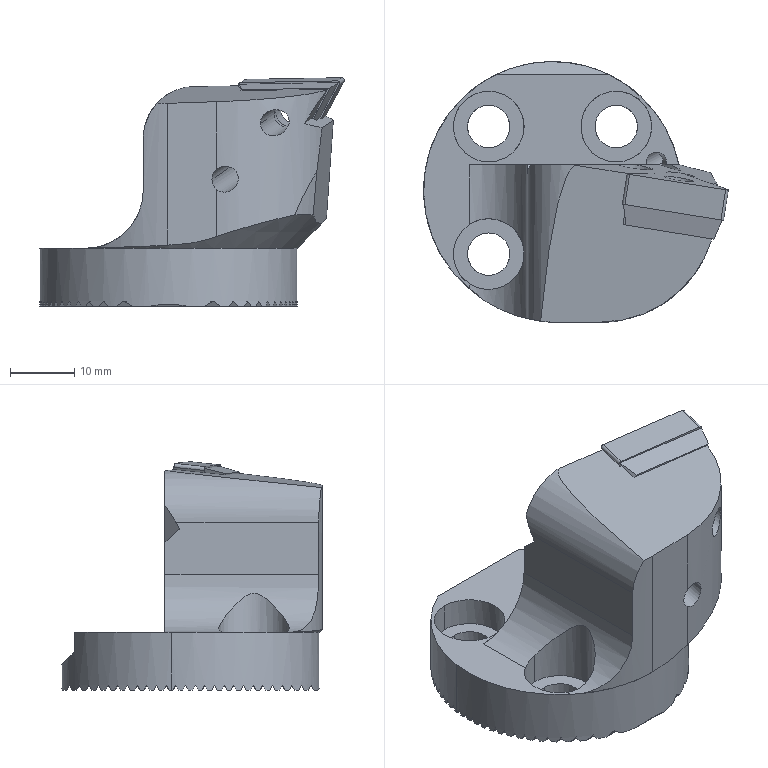NC program | Mastercam | posted with a generic post
Lines 6760 to 8002 of 11065:
(6 FEMR |TOOL - 5|DIA. OFF. - 5|LEN. - 5|TOOL DIA. - 6.)
N3668 T5 M6
N3670 G0 G54 G90 X39.195 Y22.78 C9. B-84. S3500 M3
N3672 G43 H5 Z49.995
N3674 Z1.995
N3676 G1 Z.245 F2000.
N3678 X38.335 Y23.239 Z.094 F1500.
N3680 G3 X37.724 Y23.398 Z-.005 I-.635 J-1.191
N3682 G1 X37.408 Y23.403
N3684 X37.341 Y23.163
N3686 G3 X37.182 Y21.033 I16.83 J-2.327
N3688 X37.053 Y14.522 I744.923 J-18.08
N3690 G1 X37.263 Y14.518
N3692 X37.474 Y14.514
N3694 X37.497 Z-.002
N3696 G3 X38.823 Y15.607 Z.245 J1.35
N3698 X38.847 Y15.825 I-1.326 J.257
N3700 G1 X39.026 Y22.009 F9500.
N3702 G3 X39.027 Y22.048 I-1.349 J.039
N3704 X39.01 Y22.26 I-1.35
N3706 X37.7 Y23.398 Z-.005 I-1.333 J-.212 F1500.
N3708 G1 X37.385 Y23.404
N3710 X37.365
N3712 G3 X37.157 Y22.633 I2.482 J-1.081
N3714 X36.967 Y20.031 I22.315 J-2.94
N3716 X36.875 Y15.018 I225.707 J-6.634
N3718 X36.908 Y14.704 I5.723 J.429
N3720 G1 X36.925 Y14.524
N3722 X37.346 Y14.517
N3724 X37.369 Z-.002
N3726 X37.633 Y14.543 Z.033
N3728 X37.887 Y14.62 Z.069
N3730 X38.121 Y14.746 Z.104
N3732 X38.326 Y14.915 Z.139
N3734 X38.493 Y15.12 Z.174
N3736 X38.618 Y15.355 Z.21
N3738 X38.694 Y15.609 Z.245
N3740 G3 X38.718 Y15.809 I-1.326 J.257 F9500.
N3742 G1 X38.98 Y21.992
N3744 G3 X38.981 Y22.049 I-1.348 J.057
N3746 X38.965 Y22.26 I-1.349
N3748 X37.655 Y23.399 Z-.005 I-1.333 J-.211 F1500.
N3750 G1 X37.339 Y23.404
N3752 X37.314 Y23.405
N3754 G3 X37.029 Y22.547 I2.55 J-1.324
N3756 X36.784 Y20.027 I17.143 J-2.938
N3758 X36.693 Y15.501 I112.328 J-4.526
N3760 G1 Y15.409
N3762 G3 X36.807 Y14.526 I4.202 J.095
N3764 G1 X37.018 Y14.522
N3766 X37.228 Y14.519
N3768 X37.252 Z-.002
N3770 G3 X38.577 Y15.611 Z.245 J1.35
N3772 X38.6 Y15.797 I-1.325 J.258 F9500.
N3774 G1 X38.926 Y21.979
N3776 G3 X38.928 Y22.05 I-1.349 J.071
N3778 X38.911 Y22.261 I-1.351
N3780 X37.601 Y23.4 Z-.005 I-1.334 J-.211 F1500.
N3782 G1 X37.285 Y23.405
N3784 X37.256 Y23.406
N3786 G3 X36.928 Y22.594 I2.236 J-1.377
N3788 X36.626 Y20.376 I12.079 J-2.771
N3790 X36.503 Y16.145 I72.788 J-4.231
N3792 X36.504 Y15.803 I72.911
N3794 X36.694 Y14.528 I4.559 J.028
N3796 G1 X36.905 Y14.524
N3798 X37.115 Y14.521
N3800 X37.139 Z-.002
N3802 G3 X38.464 Y15.613 Z.245 J1.349
N3804 X38.486 Y15.788 I-1.325 J.257 F9500.
N3806 G1 X38.865 Y21.968
N3808 G3 X38.868 Y22.051 I-1.347 J.083
N3810 X38.851 Y22.262 I-1.35
N3812 X37.542 Y23.401 Z-.005 I-1.333 J-.211 F1500.
N3814 G1 X37.226 Y23.406
N3816 X37.194 Y23.407
N3818 G3 X36.83 Y22.633 I2.017 J-1.424
N3820 X36.466 Y20.502 I9.938 J-2.789
N3822 X36.318 Y16.715 I48.508 J-3.787
N3824 X36.324 Y16.008 I48.656
N3826 X36.49 Y14.817 I5.524 J.16
N3828 G2 X36.584 Y14.53 I-6.781 J-2.398
N3830 G1 X36.795 Y14.526
N3832 X37.005 Y14.523
N3834 X37.029 Z-.002
N3836 G3 X38.354 Y15.615 Z.245 J1.349
N3838 X38.375 Y15.779 I-1.325 J.257 F9500.
N3840 G1 X38.802 Y21.959
N3842 G3 X38.805 Y22.052 I-1.347 J.093
N3844 X38.788 Y22.263 I-1.35
N3846 X37.479 Y23.402 Z-.005 I-1.333 J-.211 F1500.
N3848 G1 X37.163 Y23.408
N3850 X37.129
N3852 G3 X36.733 Y22.669 I1.839 J-1.46
N3854 X36.312 Y20.613 I8.505 J-2.813
N3856 X36.134 Y17.034 I35.883 J-3.579
N3858 X36.144 Y16.196 I36.061
N3860 X36.381 Y14.772 I5.219 J.137
N3862 G1 X36.476 Y14.532
N3864 X36.897 Y14.525
N3866 X36.92 Y14.524 Z-.002
N3868 G3 X38.246 Y15.617 Z.245 J1.35
N3870 X38.267 Y15.772 I-1.326 J.257 F9500.
N3872 G1 X38.735 Y21.951
N3874 G3 X38.739 Y22.053 I-1.346 J.102
N3876 X38.722 Y22.265 I-1.35
N3878 X37.413 Y23.403 Z-.005 I-1.333 J-.212 F1500.
N3880 G1 X37.097 Y23.409
N3882 X37.061
N3884 G3 X36.639 Y22.702 I1.685 J-1.485
N3886 X36.164 Y20.713 I7.489 J-2.841
N3888 X35.954 Y17.323 I27.281 J-3.39
N3890 X35.977 Y16.2 I27.491
N3892 X36.253 Y14.788 I4.982 J.242
N3894 G2 X36.368 Y14.534 I-8.619 J-4.061
N3896 G1 X36.579 Y14.53
N3898 X36.789 Y14.526
N3900 X36.813 Z-.002
N3902 G3 X38.138 Y15.619 Z.245 J1.35
N3904 X38.158 Y15.766 I-1.325 J.257 F9500.
N3906 G1 X38.666 Y21.944
N3908 G3 X38.671 Y22.055 I-1.345 J.111
N3910 X38.654 Y22.266 I-1.35
N3912 X37.344 Y23.404 Z-.005 I-1.333 J-.211 F1500.
N3914 G1 X37.029 Y23.41
N3916 X36.991 Y23.411
N3918 G3 X36.545 Y22.733 I1.555 J-1.509
N3920 X36.02 Y20.805 I6.732 J-2.872
N3922 X35.775 Y17.456 I22.746 J-3.349
N3924 X35.801 Y16.362 I22.991
N3926 X36.127 Y14.801 I4.97 J.225
N3928 X36.262 Y14.536 I5.706 J2.736
N3930 G1 X36.472 Y14.532
N3932 X36.683 Y14.528
N3934 X36.706 Z-.002
N3936 G3 X38.032 Y15.62 Z.245 J1.35
N3938 X38.051 Y15.76 I-1.326 J.258 F9500.
N3940 G1 X38.595 Y21.937
N3942 G3 X38.6 Y22.056 I-1.345 J.119
N3944 X38.584 Y22.267 I-1.35
N3946 X37.274 Y23.406 Z-.005 I-1.334 J-.211 F1500.
N3948 G1 X36.958 Y23.411
N3950 X36.919 Y23.412
N3952 G3 X36.453 Y22.763 I1.444 J-1.529
N3954 X35.88 Y20.891 I6.133 J-2.903
N3956 X35.6 Y17.599 I19.196 J-3.292
N3958 X35.639 Y16.351 I19.476
N3960 X36.002 Y14.812 I4.768 J.311
N3962 X36.039 Y14.74 I1.147 J.55
N3964 X36.225 Y14.536 I.525 J.292
N3966 G1 X36.436 Y14.533
N3968 X36.459 Z-.002
N3970 G3 X37.784 Y15.625 Z.245 J1.349
N3972 X37.8 Y15.726 I-1.325 J.257 F9500.
N3974 G1 X38.519 Y21.901
N3976 G3 X38.528 Y22.057 I-1.341 J.156
N3978 X38.512 Y22.268 I-1.35
N3980 X37.202 Y23.407 Z-.005 I-1.334 J-.211 F1500.
N3982 G1 X36.886 Y23.412
N3984 X36.845 Y23.413
N3986 G3 X36.361 Y22.792 I1.332 J-1.536
N3988 X35.743 Y20.973 I5.644 J-2.932
N3990 X35.425 Y17.675 I16.95 J-3.298
N3992 X35.466 Y16.496 I17.268
N3994 X35.82 Y14.952 I4.95 J.325
N3996 X35.95 Y14.731 I1.379 J.659
N3998 X36.162 Y14.537 I.499 J.333
N4000 G1 X36.372 Y14.534
N4002 X36.396 Z-.002
N4004 G3 X37.721 Y15.626 Z.245 J1.349
N4006 X37.737 Y15.73 I-1.325 J.257 F9500.
N4008 G1 X38.445 Y21.904
N4010 G3 X38.454 Y22.058 I-1.341 J.154
N4012 X38.438 Y22.27 I-1.35
N4014 X37.128 Y23.408 Z-.005 I-1.334 J-.212 F1500.
N4016 G1 X36.812 Y23.414
N4018 X36.769
N4020 G3 X36.208 Y22.715 I1.314 J-1.627
N4022 X35.539 Y20.717 I6.131 J-3.164
N4024 X35.255 Y17.774 I15.082 J-2.943
N4026 X35.31 Y16.474 I15.366
N4028 X35.652 Y15.063 I4.788 J.415
N4030 X35.99 Y14.606 I.996 J.383
N4032 X36.128 Y14.538 I.331 J.5
N4034 G1 X36.137 Y14.566 Z-.001
N4036 X36.682 Y16.34 Z.245
N4038 X38.319 Y21.663 F9500.
N4040 G3 X38.379 Y22.06 I-1.29 J.397
N4042 X38.362 Y22.271 I-1.35
N4044 X37.052 Y23.409 Z-.005 I-1.333 J-.211 F1500.
N4046 G1 X36.736 Y23.415
N4048 X36.691 Y23.416
N4050 G3 X36.115 Y22.746 I1.208 J-1.623
N4052 X35.403 Y20.799 I5.691 J-3.183
N4054 X35.087 Y17.845 I13.643 J-2.954
N4056 X35.157 Y16.449 I13.959
N4058 X35.569 Y14.999 I4.139 J.391
N4060 X35.898 Y14.611 I.953 J.474
N4062 X36.073 Y14.539 I.312 J.512
N4064 G2 X36.104 Y14.661 Z.012 I1.322 J-.272
N4066 G1 X36.618 Y16.343 Z.245
N4068 X38.242 Y21.667 F9500.
N4070 G3 X38.301 Y22.061 I-1.291 J.394
N4072 X38.285 Y22.272 I-1.35
N4074 X36.975 Y23.411 Z-.005 I-1.334 J-.211 F1500.
N4076 G1 X36.659 Y23.416
N4078 X36.612 Y23.417
N4080 G3 X36.022 Y22.777 I1.245 J-1.739
N4082 X35.27 Y20.878 I5.309 J-3.2
N4084 X34.921 Y17.884 I12.673 J-2.994
N4086 X34.987 Y16.578 I13.022
N4088 X35.401 Y15.092 I4.356 J.414
N4090 X35.81 Y14.605 I1.088 J.497
N4092 X35.98 Y14.541 I.294 J.523
N4094 G2 X36.017 Y14.689 Z.016 I1.327 J-.249
N4096 G1 X36.526 Y16.344 Z.245
N4098 X38.163 Y21.665 F9500.
N4100 G3 X38.223 Y22.062 I-1.291 J.397
N4102 X38.206 Y22.274 I-1.351
N4104 X36.896 Y23.412 Z-.005 I-1.334 J-.212 F1500.
N4106 G1 X36.58 Y23.418
N4108 X36.531 Y23.419
N4110 G3 X35.861 Y22.706 I1.286 J-1.879
N4112 X35.099 Y20.794 I5.44 J-3.276
N4114 X34.757 Y17.944 I11.709 J-2.85
N4116 X34.838 Y16.55 I12.051
N4118 X35.281 Y15.094 I4.178 J.474
N4120 X35.722 Y14.595 I1.105 J.533
N4122 X35.867 Y14.542 I.276 J.533
N4124 G2 X35.903 Y14.684 Z.015 I1.324 J-.26
N4126 G1 X36.421 Y16.344 Z.245
N4128 X38.081 Y21.662 F9500.
N4130 G3 X38.142 Y22.064 I-1.289 J.402
N4132 X38.125 Y22.275 I-1.35
N4134 X36.816 Y23.414 Z-.005 I-1.333 J-.211 F1500.
N4136 G1 X36.5 Y23.419
N4138 X36.448 Y23.42
N4140 G3 X35.698 Y22.636 I1.335 J-2.027
N4142 X34.89 Y20.549 I5.681 J-3.402
N4144 X34.596 Y17.978 I11.096 J-2.571
N4146 X34.671 Y16.67 I11.39
N4148 X35.163 Y15.089 I4.304 J.473
N4150 X35.626 Y14.594 I1.103 J.566
N4152 X35.79 Y14.544 I.254 J.543
N4154 G2 X35.839 Y14.762 Z.025 I1.337 J-.185
N4156 G1 X36.335 Y16.347 Z.245
N4158 X37.998 Y21.662 F9500.
N4160 G3 X38.06 Y22.065 I-1.288 J.403
N4162 X38.043 Y22.276 I-1.35
N4164 X36.734 Y23.415 Z-.005 I-1.333 J-.211 F1500.
N4166 G1 X36.418 Y23.421
N4168 X36.364
N4170 G3 X35.602 Y22.671 I1.302 J-2.084
N4172 X34.757 Y20.63 I5.341 J-3.407
N4174 X34.435 Y18.029 I10.353 J-2.601
N4176 X34.526 Y16.636 I10.675
N4178 X35.049 Y15.077 I4.19 J.536
N4180 X35.529 Y14.59 I1.115 J.621
N4182 X35.698 Y14.545 I.236 J.552
N4184 G2 X35.754 Y14.813 Z.032 I1.343 J-.138
N4186 G1 X36.238 Y16.35 Z.245
N4188 X37.914 Y21.66 F9500.
N4190 G3 X37.977 Y22.067 I-1.287 J.407
N4192 X37.96 Y22.278 I-1.35
N4194 X36.65 Y23.416 Z-.005 I-1.333 J-.211 F1500.
N4196 G1 X36.334 Y23.422
N4198 X36.278 Y23.423
N4200 G3 X35.506 Y22.705 I1.218 J-2.085
N4202 X34.627 Y20.71 I5.032 J-3.408
N4204 X34.278 Y18.056 I9.904 J-2.654
N4206 X34.361 Y16.748 I10.253
N4208 X34.881 Y15.148 I4.427 J.553
N4210 X35.259 Y14.689 I1.565 J.907
N4212 X35.549 Y14.548 I.398 J.449
N4214 G2 X35.597 Y14.746 Z.022 I1.332 J-.217
N4216 G1 X36.113 Y16.346 Z.245
N4218 X37.826 Y21.653 F9500.
N4220 G3 X37.891 Y22.068 I-1.284 J.415
N4222 X37.875 Y22.279 I-1.349
N4224 X36.565 Y23.418 Z-.005 I-1.333 J-.211 F1500.
N4226 G1 X36.249 Y23.423
N4228 X36.19 Y23.424
N4230 G3 X35.337 Y22.64 I1.223 J-2.187
N4232 X34.456 Y20.63 I5.151 J-3.455
N4234 X34.12 Y18.098 I9.386 J-2.532
N4236 X34.22 Y16.707 I9.722
N4238 X34.766 Y15.13 I4.322 J.613
N4240 X35.143 Y14.689 I1.556 J.949
N4242 X35.481 Y14.549 I.388 J.458
N4244 G2 X35.543 Y14.863 Z.038 I1.347 J-.101
N4246 G1 X36.024 Y16.352 Z.245
N4248 X37.739 Y21.654 F9500.
N4250 G3 X37.805 Y22.07 I-1.284 J.416
N4252 X37.788 Y22.281 I-1.35
N4254 X36.478 Y23.419 Z-.005 I-1.333 J-.211 F1500.
N4256 G1 X36.163 Y23.425
N4258 X36.101 Y23.426
N4260 G3 X35.239 Y22.676 I1.109 J-2.145
N4262 X34.327 Y20.707 I4.888 J-3.459
N4264 X33.966 Y18.118 I9.105 J-2.589
N4266 X34.057 Y16.811 I9.466
N4268 X34.653 Y15.11 I4.342 J.566
N4270 X35.048 Y14.673 I1.413 J.88
N4272 X35.4 Y14.551 I.362 J.478
N4274 G1 X35.423 Z-.002
N4276 X35.687 Y14.577 Z.033
N4278 X35.941 Y14.654 Z.069
N4280 X36.175 Y14.78 Z.104
N4282 X36.38 Y14.949 Z.139
N4284 X36.547 Y15.154 Z.174
N4286 X36.672 Y15.389 Z.21
N4288 X36.748 Y15.643 Z.245
N4290 G3 X36.758 Y15.696 I-1.326 J.257 F9500.
N4292 G1 X37.701 Y21.867
N4294 G3 X37.717 Y22.071 I-1.334 J.204
N4296 X37.7 Y22.282 I-1.35
N4298 X36.39 Y23.421 Z-.005 I-1.333 J-.211 F1500.
N4300 G1 X36.075 Y23.427
N4302 X36.01 Y23.428
N4304 G3 X35.141 Y22.71 I1.012 J-2.111
N4306 X34.2 Y20.781 I4.654 J-3.463
N4308 X33.812 Y18.151 I8.73 J-2.63
N4310 X33.919 Y16.763 I9.118
N4312 X34.541 Y15.087 I4.244 J.621
N4314 X34.923 Y14.677 I1.437 J.957
N4316 X35.278 Y14.553 I.366 J.476
N4318 G1 X35.302 Z-.002
N4320 G3 X36.627 Y15.645 Z.245 J1.35
N4322 X36.635 Y15.692 I-1.325 J.258 F9500.
N4324 G1 X37.61 Y21.862
N4326 G3 X37.627 Y22.073 I-1.333 J.211
N4328 X37.61 Y22.284 I-1.35
N4330 X36.3 Y23.423 Z-.005 I-1.333 J-.211 F1500.
N4332 G1 X35.985 Y23.428
N4334 X35.857 Y23.407
N4336 G3 X34.89 Y22.547 I1.237 J-2.364
N4338 X33.943 Y20.389 I5.295 J-3.609
N4340 X33.657 Y18.182 I8.386 J-2.207
N4342 X33.783 Y16.712 I8.672
N4344 X34.43 Y15.062 I4.142 J.673
N4346 X34.809 Y14.672 I1.396 J.974
N4348 X35.154 Y14.555 I.355 J.483
N4350 G1 X35.364 Y14.551
N4352 X35.388 Z-.002
N4354 G3 X36.713 Y15.643 Z.245 J1.35
N4356 X36.727 Y15.728 I-1.325 J.258 F9500.
N4358 G1 X37.524 Y21.901
N4360 G3 X37.535 Y22.074 I-1.339 J.173
N4362 X37.519 Y22.286 I-1.35
N4364 X36.209 Y23.424 Z-.005 I-1.334 J-.212 F1500.
N4366 G1 X35.893 Y23.43
N4368 X35.763 Y23.411
N4370 G3 X34.788 Y22.584 I1.13 J-2.322
N4372 X33.813 Y20.464 I5.056 J-3.608
N4374 X33.508 Y18.206 I8.192 J-2.258
N4376 X33.65 Y16.657 I8.497
N4378 X34.322 Y15.035 I4.041 J.723
N4380 X34.692 Y14.667 I1.342 J.979
N4382 X35.028 Y14.557 I.346 J.49
N4384 G1 X35.238 Y14.553
N4386 X35.262 Z-.002
N4388 G3 X36.587 Y15.646 Z.245 J1.35
N4390 X36.6 Y15.723 I-1.325 J.257 F9500.
N4392 G1 X37.43 Y21.896
N4394 G3 X37.442 Y22.076 I-1.338 J.18
N4396 X37.426 Y22.287 I-1.35
N4398 X36.116 Y23.426 Z-.005 I-1.334 J-.211 F1500.
N4400 G1 X35.8 Y23.431
N4402 X35.666 Y23.414
N4404 G3 X34.685 Y22.619 I1.03 J-2.274
N4406 X33.684 Y20.534 I4.836 J-3.604
N4408 X33.358 Y18.23 I7.983 J-2.304
N4410 X33.52 Y16.599 I8.309
N4412 X34.215 Y15.006 I3.936 J.769
N4414 X34.842 Y14.569 I.945 J.689
N4416 X35.063 Y14.552 I.221 J1.406
N4418 X35.155 Y14.555 J1.423
N4420 G1 X35.179 Z-.002
N4422 G3 X36.504 Y15.647 Z.245 J1.35
N4424 X36.517 Y15.727 I-1.325 J.258 F9500.
N4426 G1 X37.336 Y21.9
N4428 G3 X37.348 Y22.078 I-1.338 J.178
N4430 X37.331 Y22.289 I-1.35
N4432 X36.021 Y23.427 Z-.005 I-1.333 J-.211 F1500.
N4434 G1 X35.706 Y23.433
N4436 X35.567 Y23.417
N4438 G3 X34.58 Y22.651 I.957 J-2.253
N4440 X33.555 Y20.6 I4.636 J-3.597
N4442 X33.206 Y18.247 I7.769 J-2.353
N4444 X33.359 Y16.68 I8.118
N4446 X34.04 Y15.063 I4.103 J.775
N4448 X34.215 Y14.903 I.484 J.354
N4450 G1 X34.396 Y14.794
N4452 G3 X34.842 Y14.569 I.899 J1.226
N4454 X34.955 Y14.558 Z.01 I.113 J.589
N4456 X35.548 Y15.068 Z.123 J.6
N4458 G1 X35.687 Y15.977 Z.245
N4460 X36.607 Y21.987 F9500.
N4462 X36.689 Y22.523 Z.173 F1500.
N4464 G3 X36.698 Y22.642 Z.157 I-.778 J.119
N4466 X35.925 Y23.429 Z-.005 I-.787
N4468 G1 X35.609 Y23.435
N4470 X35.465 Y23.42
N4472 G3 X34.473 Y22.681 I.887 J-2.225
N4474 X33.427 Y20.661 I4.426 J-3.574
N4476 X33.06 Y18.266 I7.623 J-2.395
N4478 X33.232 Y16.612 I7.99
N4480 X33.813 Y15.202 I4.108 J.869
N4482 X33.992 Y15.037 I.488 J.349
N4484 G1 X34.173 Y14.928
N4486 X34.353 Y14.82
N4488 G3 X35.049 Y14.627 Z.092 I.696 J1.157
N4490 X36.067 Y15.092 Z.245 J1.35
N4492 X36.388 Y15.812 I-1.018 J.885 F9500.
N4494 G1 X37.142 Y21.916
N4496 G3 X37.152 Y22.081 I-1.34 J.165
N4498 X37.135 Y22.292 I-1.35
N4500 X35.825 Y23.431 Z-.005 I-1.333 J-.211 F1500.
N4502 G1 X35.51 Y23.436
N4504 X35.362 Y23.423
N4506 G3 X34.367 Y22.711 I.821 J-2.198
N4508 X33.299 Y20.721 I4.267 J-3.572
N4510 X32.912 Y18.275 I7.542 J-2.446
N4512 X33.073 Y16.685 I7.929
N4514 X33.598 Y15.341 I4.076 J.817
N4516 X33.788 Y15.16 I.499 J.333
N4518 G1 X33.969 Y15.051
N4520 X34.149 Y14.943
N4522 G3 X34.844 Y14.75 Z.092 I.695 J1.157
N4524 X35.863 Y15.214 Z.245 J1.35
N4526 X36.181 Y15.909 I-1.019 J.886 F9500.
N4528 G1 X37.036 Y21.892
N4530 G3 X37.05 Y22.083 I-1.336 J.191
N4532 X37.033 Y22.294 I-1.35
N4534 X35.723 Y23.433 Z-.005 I-1.333 J-.211 F1500.
N4536 G1 X35.408 Y23.438
N4538 X35.257 Y23.427
N4540 G3 X34.261 Y22.741 I.758 J-2.169
N4542 X33.172 Y20.78 I4.134 J-3.578
N4544 X32.764 Y18.294 I7.376 J-2.486
N4546 X32.948 Y16.614 I7.784
N4548 X33.405 Y15.458 I3.742 J.811
N4550 X33.596 Y15.275 I.5 J.332
N4552 G1 X33.776 Y15.167
N4554 X33.956 Y15.058
N4556 G3 X34.652 Y14.865 Z.092 I.696 J1.158
N4558 X35.671 Y15.33 Z.245 J1.351
N4560 X35.985 Y16.001 I-1.019 J.886 F9500.
N4562 G1 X36.929 Y21.87
N4564 G3 X36.946 Y22.085 I-1.333 J.215
N4566 X36.929 Y22.296 I-1.35
N4568 X35.62 Y23.434 Z-.005 I-1.333 J-.211 F1500.
N4570 G1 X35.304 Y23.44
N4572 X35.149 Y23.43
N4574 G3 X34.15 Y22.767 I.702 J-2.141
N4576 X33.044 Y20.832 I4.009 J-3.577
N4578 X32.618 Y18.311 I7.245 J-2.521
N4580 X32.825 Y16.538 I7.671
N4582 X33.209 Y15.585 I3.395 J.813
N4584 X33.41 Y15.387 I.51 J.316
N4586 G1 X33.591 Y15.278
N4588 X33.771 Y15.17
N4590 G3 X34.466 Y14.977 Z.092 I.695 J1.157
N4592 X35.485 Y15.441 Z.245 J1.35
N4594 X35.795 Y16.091 I-1.019 J.886 F9500.
N4596 G1 X36.82 Y21.85
N4598 G3 X36.841 Y22.087 I-1.33 J.237
N4600 X36.824 Y22.298 I-1.351
N4602 X35.514 Y23.436 Z-.005 I-1.334 J-.211 F1500.
N4604 G1 X35.198 Y23.442
N4606 X34.992 Y23.42
N4608 G3 X33.977 Y22.726 I.778 J-2.227
N4610 X32.83 Y20.623 I4.142 J-3.625
N4612 X32.473 Y18.317 I7.268 J-2.306
N4614 X32.66 Y16.634 I7.625
N4616 X33.028 Y15.695 I3.285 J.746
N4618 X33.231 Y15.494 I.512 J.314
N4620 G1 X33.411 Y15.386
N4622 X33.592 Y15.278
N4624 G3 X34.287 Y15.085 Z.092 I.695 J1.157
N4626 X35.306 Y15.549 Z.245 J1.35
N4628 X35.612 Y16.177 I-1.019 J.886 F9500.
N4630 G1 X36.712 Y21.83
N4632 G3 X36.737 Y22.088 I-1.325 J.258
N4634 X36.721 Y22.299 I-1.35
N4636 X35.411 Y23.438 Z-.005 I-1.334 J-.211 F1500.
N4638 X35.095 Y23.444 I-.876 J-41.251
N4640 G1 X35.089
N4642 G3 X34.798 Y23.368 J-.6
N4644 G1 X34.614 Y23.266
N4646 G3 X33.509 Y22.311 I1.244 J-2.557
N4648 X32.457 Y19.71 I5.355 J-3.678
N4650 X32.327 Y18.33 I7.285 J-1.38
N4652 X32.55 Y16.528 I7.415
N4654 X32.858 Y15.794 I2.667 J.686
N4656 X33.057 Y15.599 I.508 J.319
N4658 G1 X33.237 Y15.491
N4660 X33.417 Y15.382
N4662 G3 X34.113 Y15.189 Z.092 I.696 J1.158
N4664 X35.132 Y15.654 Z.245 J1.351
N4666 X35.436 Y16.274 I-1.019 J.886 F9500.
N4668 G1 X36.543 Y21.793
N4670 G3 X36.569 Y22.059 I-1.323 J.266
N4672 X36.269 Y22.908 I-1.349
N4674 X35.22 Y23.409 Z.086 I-1.049 J-.849 F1500.
N4676 X34.565 Y23.239 Z-.005 J-1.35
N4678 G1 X34.289 Y23.086
N4680 G3 X33.352 Y22.269 I1.152 J-2.265
N4682 X32.338 Y19.846 I5.139 J-3.576
N4684 X32.184 Y18.342 I7.254 J-1.504
N4686 X32.376 Y16.666 I7.408
N4688 X32.682 Y15.904 I2.71 J.648
N4690 X32.886 Y15.702 I.513 J.312
N4692 G1 X33.066 Y15.593
N4694 X33.247 Y15.485
N4696 G3 X33.942 Y15.292 Z.092 I.695 J1.157
N4698 X34.961 Y15.756 Z.245 J1.35
N4700 X35.266 Y16.377 I-1.019 J.886 F9500.
N4702 G1 X36.328 Y21.674
N4704 G3 X36.354 Y21.939 I-1.323 J.265
N4706 X36.054 Y22.789 I-1.349
N4708 X35.005 Y23.289 Z.086 I-1.049 J-.85 F1500.
N4710 X34.35 Y23.12 Z-.005 J-1.35
N4712 G1 X34.074 Y22.967
N4714 G3 X33.125 Y22.123 I1.108 J-2.201
N4716 X32.161 Y19.681 I5.217 J-3.472
N4718 X32.038 Y18.358 I7.046 J-1.323
N4720 X32.235 Y16.685 I7.169
N4722 X32.52 Y15.996 I2.454 J.611
N4724 X32.719 Y15.802 I.508 J.32
N4726 G1 X32.899 Y15.694
N4728 X33.08 Y15.585
N4730 G3 X33.775 Y15.392 Z.092 I.695 J1.157
N4732 X34.794 Y15.857 Z.245 J1.35
N4734 X35.1 Y16.485 I-1.019 J.885 F9500.
N4736 G1 X36.085 Y21.546
N4738 G3 X36.11 Y21.804 I-1.325 J.258
N4740 X35.809 Y22.653 I-1.35
N4742 X34.76 Y23.154 Z.086 I-1.049 J-.849 F1500.
N4744 X34.105 Y22.984 Z-.005 J-1.35
N4746 G1 X33.829 Y22.831
N4748 G3 X32.975 Y22.077 I1.035 J-2.034
N4750 X32.014 Y19.669 I4.98 J-3.381
N4752 X31.893 Y18.378 I6.836 J-1.291
N4754 X32.097 Y16.707 I6.957
N4756 X32.35 Y16.104 I2.387 J.648
N4758 X32.554 Y15.901 I.513 J.311
N4760 G1 X32.735 Y15.792
N4762 X32.915 Y15.684
N4764 G3 X33.611 Y15.491 Z.092 I.696 J1.157
N4766 X34.629 Y15.956 Z.245 J1.35
N4768 X34.935 Y16.579 I-1.018 J.885 F9500.
N4770 G1 X35.899 Y21.438
N4772 G3 X35.925 Y21.701 I-1.324 J.263
N4774 X35.624 Y22.55 I-1.35
N4776 X34.575 Y23.051 Z.086 I-1.049 J-.849 F1500.
N4778 X33.92 Y22.882 Z-.005 J-1.35
N4780 G1 X33.644 Y22.729
N4782 G3 X32.754 Y21.929 I1.028 J-2.04
N4784 X31.843 Y19.503 I5.08 J-3.293
N4786 X31.75 Y18.385 I6.662 J-1.118
N4788 X31.926 Y16.852 I6.755
N4790 X32.183 Y16.211 I2.482 J.624
N4792 X32.392 Y15.998 I.518 J.302
N4794 G1 X32.573 Y15.89
N4796 X32.753 Y15.781
N4798 G3 X33.449 Y15.588 Z.092 I.696 J1.158
N4800 X34.468 Y16.053 Z.245 J1.351
N4802 X34.774 Y16.681 I-1.019 J.886 F9500.
N4804 G1 X35.676 Y21.319
N4806 G3 X35.701 Y21.577 I-1.325 J.258
N4808 X35.4 Y22.426 I-1.35
N4810 X34.351 Y22.927 Z.086 I-1.049 J-.849 F1500.
N4812 X33.696 Y22.758 Z-.005 J-1.35
N4814 G1 X33.42 Y22.604
N4816 G3 X32.591 Y21.859 I1.006 J-1.95
N4818 X31.718 Y19.607 I4.804 J-3.159
N4820 X31.609 Y18.403 I6.571 J-1.204
N4822 X31.766 Y16.964 I6.68
N4824 X32.021 Y16.311 I2.498 J.6
N4826 X32.233 Y16.094 I.521 J.297
N4828 G1 X32.414 Y15.986
N4830 X32.594 Y15.877
N4832 G3 X33.289 Y15.684 Z.092 I.695 J1.157
N4834 X34.308 Y16.149 Z.245 J1.35
N4836 X34.614 Y16.773 I-1.019 J.885 F9500.
N4838 G1 X35.491 Y21.213
N4840 G3 X35.517 Y21.475 I-1.324 J.262
N4842 X35.216 Y22.324 I-1.35
N4844 X34.167 Y22.825 Z.086 I-1.049 J-.849 F1500.
N4846 X33.512 Y22.655 Z-.005 J-1.35
N4848 G1 X33.236 Y22.502
N4850 G3 X32.424 Y21.777 I.945 J-1.875
N4852 X31.566 Y19.545 I4.683 J-3.079
N4854 X31.467 Y18.427 I6.233 J-1.118
N4856 X31.642 Y16.95 I6.332
N4858 X31.873 Y16.391 I2.183 J.576
N4860 X32.077 Y16.188 I.513 J.311
N4862 G1 X32.257 Y16.079
N4864 X32.438 Y15.971
N4866 G3 X33.133 Y15.778 Z.092 I.695 J1.157
N4868 X34.152 Y16.242 Z.245 J1.35
N4870 X34.457 Y16.863 I-1.019 J.886 F9500.
N4872 G1 X35.306 Y21.108
N4874 G3 X35.332 Y21.373 I-1.324 J.265
N4876 X35.032 Y22.222 I-1.35
N4878 X33.982 Y22.723 Z.085 I-1.05 J-.849 F1500.
N4880 X33.328 Y22.553 Z-.005 J-1.35
N4882 G1 X33.052 Y22.4
N4884 G3 X32.245 Y21.677 I.923 J-1.842
N4886 X31.412 Y19.454 I4.614 J-2.997
N4888 X31.327 Y18.443 I5.998 J-1.011
N4890 X31.493 Y17.033 I6.083
N4892 X31.719 Y16.484 I2.128 J.555
N4894 X31.923 Y16.28 I.513 J.311
N4896 G1 X32.103 Y16.172
N4898 X32.284 Y16.064
N4900 G3 X32.979 Y15.871 Z.092 I.695 J1.157
N4902 X33.998 Y16.335 Z.245 J1.35
N4904 X34.302 Y16.954 I-1.019 J.886 F9500.
N4906 G1 X35.117 Y21.002
N4908 G3 X35.143 Y21.268 I-1.324 J.266
N4910 X34.842 Y22.117 I-1.35
N4912 X33.793 Y22.618 Z.086 I-1.049 J-.849 F1500.
N4914 X33.139 Y22.449 Z-.005 J-1.35
N4916 G1 X32.863 Y22.295
N4918 G3 X32.068 Y21.577 I.922 J-1.818
N4920 X31.259 Y19.363 I4.543 J-2.915
N4922 X31.188 Y18.458 I5.721 J-.905
N4924 X31.346 Y17.114 I5.792
N4926 X31.555 Y16.594 I2.111 J.548
N4928 X31.77 Y16.372 I.524 J.292
N4930 G1 X31.951 Y16.264
N4932 X32.131 Y16.155
N4934 G3 X32.826 Y15.962 Z.092 I.695 J1.157
N4936 X33.845 Y16.427 Z.245 J1.35
N4938 X34.149 Y17.044 I-1.019 J.885 F9500.
N4940 G1 X34.932 Y20.897
N4942 G3 X34.959 Y21.166 I-1.323 J.269
N4944 X34.658 Y22.015 I-1.35
N4946 X33.609 Y22.516 Z.086 I-1.049 J-.849 F1500.
N4948 X32.955 Y22.346 Z-.005 J-1.35
N4950 G1 X32.678 Y22.193
N4952 G3 X31.888 Y21.469 I.941 J-1.82
N4954 X31.089 Y19.113 I4.601 J-2.873
N4956 X31.049 Y18.466 I5.219 J-.647
N4958 X31.235 Y17.08 I5.259
N4960 X31.406 Y16.684 I1.906 J.584
N4962 X31.62 Y16.462 I.523 J.293
N4964 G1 X31.801 Y16.354
N4966 X31.981 Y16.245
N4968 G3 X32.676 Y16.052 Z.092 I.695 J1.158
N4970 X33.695 Y16.517 Z.245 J1.351
N4972 X33.999 Y17.132 I-1.019 J.886 F9500.
N4974 G1 X34.748 Y20.793
N4976 G3 X34.775 Y21.064 I-1.323 J.271
N4978 X34.474 Y21.913 I-1.35
N4980 X33.425 Y22.414 Z.086 I-1.049 J-.849 F1500.
N4982 X32.77 Y22.244 Z-.005 J-1.35
N4984 G1 X32.494 Y22.091
N4986 G3 X31.706 Y21.355 I.919 J-1.774
N4988 X30.942 Y19.004 I4.55 J-2.777
N4990 X30.913 Y18.476 I4.773 J-.528
N4992 X31.131 Y17.047 I4.802
N4994 X31.392 Y16.609 I1.002 J.301
N4996 X31.834 Y16.334 I1.857 J2.49
N4998 X32.529 Y16.141 Z.092 I.695 J1.157
N5000 X33.548 Y16.606 Z.245 J1.35
N5002 X33.851 Y17.22 I-1.019 J.885 F9500.
N5004 G1 X34.563 Y20.69
N5006 G3 X34.591 Y20.962 I-1.322 J.272
N5008 X34.29 Y21.811 I-1.35
N5010 X33.241 Y22.312 Z.086 I-1.049 J-.849 F1500.
N5012 X32.586 Y22.142 Z-.005 J-1.35
N5014 G1 X32.31 Y21.989
N5016 G3 X31.522 Y21.235 I.925 J-1.755
N5018 X30.785 Y18.6 I4.605 J-2.709
N5020 X30.781 Y18.424 I4.051 J-.176
N5022 X31.029 Y17.026 I4.055
N5024 X31.116 Y16.855 I1.403 J.598
N5026 X31.327 Y16.638 I.52 J.297
N5028 G1 X31.508 Y16.53
N5030 X31.688 Y16.421
N5032 G3 X32.384 Y16.228 Z.092 I.696 J1.158
N5034 X33.402 Y16.693 Z.245 J1.351
N5036 X33.706 Y17.307 I-1.018 J.886 F9500.
N5038 G1 X34.379 Y20.588
N5040 G3 X34.407 Y20.86 I-1.322 J.272
N5042 X34.106 Y21.709 I-1.35
N5044 X33.057 Y22.21 Z.086 I-1.049 J-.849 F1500.
N5046 X32.402 Y22.04 Z-.005 J-1.35
N5048 G1 X32.126 Y21.887
N5050 G3 X31.4 Y21.208 I.933 J-1.725
N5052 X30.659 Y18.767 I4.286 J-2.633
N5054 X30.649 Y18.484 I4.134 J-.283
N5056 X30.864 Y17.168 I4.144
N5058 X30.964 Y16.955 I1.528 J.588
N5060 X31.184 Y16.725 I.529 J.284
N5062 G1 X31.364 Y16.616
N5064 X31.545 Y16.508
N5066 G3 X32.24 Y16.315 Z.092 I.695 J1.157
N5068 X33.259 Y16.779 Z.245 J1.35
N5070 X33.562 Y17.394 I-1.019 J.886 F9500.
N5072 G1 X34.195 Y20.487
N5074 G3 X34.222 Y20.757 I-1.322 J.27
N5076 X33.922 Y21.607 I-1.349
N5078 X32.873 Y22.107 Z.086 I-1.049 J-.85 F1500.
N5080 X32.218 Y21.938 Z-.005 J-1.35
N5082 G1 X31.942 Y21.785
N5084 G3 X31.276 Y21.174 I.854 J-1.599
N5086 X30.54 Y18.923 I4.021 J-2.561
N5088 X30.52 Y18.525 I4.013 J-.398
N5090 X30.736 Y17.223 I4.033
N5092 X30.826 Y17.035 I1.43 J.57
N5094 X31.043 Y16.809 I.526 J.288
N5096 G1 X31.223 Y16.701
N5098 X31.404 Y16.592
N5100 G3 X32.099 Y16.399 Z.092 I.695 J1.157
N5102 X33.118 Y16.864 Z.245 J1.35
N5104 X33.422 Y17.481 I-1.019 J.885 F9500.
N5106 G1 X34.012 Y20.387
N5108 G3 X34.039 Y20.655 I-1.323 J.268
N5110 X33.738 Y21.505 I-1.35
N5112 X32.689 Y22.005 Z.086 I-1.049 J-.85 F1500.
N5114 X32.034 Y21.836 Z-.005 J-1.35
N5116 G1 X31.758 Y21.683
N5118 X31.52 Y21.54
N5120 G3 X30.752 Y20.396 I1.94 J-2.132
N5122 X30.397 Y18.594 I4.399 J-1.802
N5124 X30.491 Y17.653 I4.754
N5126 X30.69 Y17.113 I1.974 J.421
N5128 X30.905 Y16.892 I.524 J.294
N5130 G1 X31.085 Y16.784
N5132 X31.265 Y16.675
N5134 G3 X31.961 Y16.482 Z.092 I.696 J1.158
N5136 X32.98 Y16.947 Z.245 J1.351
N5138 X33.285 Y17.568 I-1.019 J.886 F9500.
N5140 G1 X33.828 Y20.289
N5142 G3 X33.854 Y20.553 I-1.324 J.264
N5144 X33.554 Y21.403 I-1.35
N5146 X32.504 Y21.904 Z.086 I-1.05 J-.85 F1500.
N5148 X31.85 Y21.734 Z-.005 J-1.351
N5150 G1 X31.574 Y21.581
N5152 X31.351 Y21.445
N5154 G3 X30.598 Y20.302 I1.942 J-2.099
N5156 X30.272 Y18.614 I4.212 J-1.688
N5158 X30.361 Y17.722 I4.538
N5160 X30.554 Y17.195 I1.919 J.404
N5162 X30.768 Y16.974 I.524 J.293
N5164 G1 X30.949 Y16.866
N5166 X31.129 Y16.757
N5168 G3 X31.825 Y16.564 Z.092 I.696 J1.157
N5170 X32.844 Y17.029 Z.245 J1.35
N5172 X33.148 Y17.649 I-1.019 J.885 F9500.
N5174 G1 X33.659 Y20.194
N5176 G3 X33.685 Y20.46 I-1.324 J.266
N5178 X33.384 Y21.309 I-1.35
N5180 X32.335 Y21.81 Z.086 I-1.049 J-.849 F1500.
N5182 X31.681 Y21.64 Z-.005 J-1.35
N5184 G1 X31.405 Y21.487
N5186 X31.197 Y21.361
N5188 G3 X30.455 Y20.231 I1.882 J-2.045
N5190 X30.149 Y18.645 I3.955 J-1.586
N5192 X30.252 Y17.71 I4.261
N5194 X30.418 Y17.28 I1.716 J.413
N5196 X30.635 Y17.054 I.526 J.289
N5198 G1 X30.815 Y16.946
N5200 X30.996 Y16.838
N5202 G3 X31.691 Y16.645 Z.092 I.695 J1.157
N5204 X32.71 Y17.109 Z.245 J1.35
N5206 X33.013 Y17.723 I-1.019 J.886 F9500.
N5208 G1 X33.502 Y20.102
N5210 G3 X33.529 Y20.373 I-1.322 J.271
N5212 X33.229 Y21.223 I-1.349
N5214 X32.18 Y21.723 Z.086 I-1.049 J-.85 F1500.
N5216 X31.525 Y21.554 Z-.005 J-1.35
N5218 G1 X31.249 Y21.401
N5220 X31.04 Y21.273
N5222 G3 X30.311 Y20.153 I1.851 J-2.001
N5224 X30.029 Y18.662 I3.803 J-1.491
N5226 X30.122 Y17.795 I4.085
N5228 X30.284 Y17.363 I1.704 J.393
N5230 X30.503 Y17.133 I.528 J.285
N5232 G1 X30.684 Y17.025
N5234 X30.864 Y16.916
N5236 G3 X31.56 Y16.723 Z.092 I.696 J1.158
N5238 X32.578 Y17.188 Z.245 J1.351
N5240 X32.881 Y17.797 I-1.018 J.886 F9500.
N5242 G1 X33.343 Y20.01
N5244 G3 X33.372 Y20.286 I-1.321 J.276
N5246 X33.071 Y21.136 I-1.35
N5248 X32.022 Y21.636 Z.086 I-1.049 J-.85 F1500.
N5250 X31.367 Y21.467 Z-.005 J-1.35
N5252 G1 X31.091 Y21.314
N5254 X30.889 Y21.19
N5256 G3 X30.172 Y20.082 I1.803 J-1.951
N5258 X29.911 Y18.679 I3.641 J-1.403
N5260 X29.993 Y17.883 I3.902
N5262 X30.153 Y17.446 I1.704 J.372
N5264 X30.375 Y17.211 I.531 J.279
N5266 G1 X30.555 Y17.102
N5268 X30.736 Y16.994
N5270 G3 X31.431 Y16.801 Z.092 I.695 J1.157
N5272 X32.45 Y17.265 Z.245 J1.35
N5274 X32.751 Y17.868 I-1.019 J.886 F9500.
N5276 G1 X33.19 Y19.919
N5278 G3 X33.22 Y20.202 I-1.32 J.283
N5280 X32.919 Y21.051 I-1.35
N5282 X31.87 Y21.552 Z.086 I-1.049 J-.849 F1500.
N5284 X31.215 Y21.382 Z-.005 J-1.35
N5286 G1 X30.939 Y21.229
N5288 X30.738 Y21.107
N5290 G3 X30.036 Y20.01 I1.764 J-1.904
N5292 X29.796 Y18.705 I3.426 J-1.305
N5294 X29.892 Y17.872 I3.666
N5296 X30.15 Y17.36 I1.071 J.22
N5298 X30.609 Y17.07 I1.616 J2.046
N5300 X31.305 Y16.877 Z.092 I.696 J1.157
N5302 X32.323 Y17.341 Z.245 J1.35
N5304 X32.623 Y17.938 I-1.018 J.886 F9500.
N5306 G1 X33.038 Y19.829
N5308 G3 X33.069 Y20.118 I-1.319 J.289
N5310 X32.768 Y20.968 I-1.35
N5312 X31.719 Y21.468 Z.086 I-1.049 J-.85 F1500.
N5314 X31.064 Y21.299 Z-.005 J-1.35
N5316 G1 X30.788 Y21.146
N5318 X30.592 Y21.026
N5320 G3 X29.903 Y19.942 I1.718 J-1.853
N5322 X29.685 Y18.728 I3.267 J-1.214
N5324 X29.792 Y17.869 I3.485
N5326 X29.897 Y17.607 I1.418 J.415
N5328 X30.125 Y17.361 I.537 J.268
N5330 G1 X30.305 Y17.252
N5332 X30.486 Y17.144
N5334 G3 X31.181 Y16.951 Z.092 I.695 J1.157
N5336 X32.2 Y17.415 Z.245 J1.35
N5338 X32.498 Y18.005 I-1.019 J.886 F9500.
N5340 G1 X32.889 Y19.74
N5342 G3 X32.922 Y20.036 I-1.317 J.296
N5344 X32.621 Y20.886 I-1.35
N5346 X31.572 Y21.386 Z.086 I-1.049 J-.85 F1500.
N5348 X30.917 Y21.217 Z-.005 J-1.35
N5350 G1 X30.641 Y21.064
N5352 X30.448 Y20.946
N5354 G3 X29.736 Y19.762 I1.751 J-1.859
N5356 X29.575 Y18.75 I3.091 J-1.012
N5358 X29.695 Y17.872 I3.252
N5360 X29.773 Y17.686 I1.327 J.446
N5362 X30.004 Y17.433 I.54 J.262
N5364 G1 X30.184 Y17.325
N5366 X30.365 Y17.216
N5368 G3 X31.06 Y17.023 Z.092 I.695 J1.158
N5370 X32.079 Y17.488 Z.245 J1.351
N5372 X32.375 Y18.069 I-1.019 J.886 F9500.
N5374 G1 X32.742 Y19.651
N5376 G3 X32.777 Y19.956 I-1.315 J.305
N5378 X32.476 Y20.806 I-1.35
N5380 X31.427 Y21.306 Z.086 I-1.049 J-.85 F1500.
N5382 X30.772 Y21.137 Z-.005 J-1.35
N5384 G1 X30.496 Y20.984
N5386 X30.306 Y20.868
N5388 G3 X29.612 Y19.7 I1.701 J-1.803
N5390 X29.468 Y18.764 I2.964 J-.936
N5392 X29.574 Y17.956 I3.108
N5394 X29.652 Y17.763 I1.331 J.425
N5396 X29.886 Y17.504 I.543 J.256
N5398 G1 X30.066 Y17.396
N5400 X30.247 Y17.287
N5402 G3 X30.942 Y17.094 Z.092 I.695 J1.158
N5404 X31.961 Y17.559 Z.245 J1.351
N5406 X32.255 Y18.131 I-1.019 J.886 F9500.
N5408 G1 X32.598 Y19.563
N5410 G3 X32.635 Y19.877 I-1.313 J.314
N5412 X32.334 Y20.727 I-1.35
N5414 X31.285 Y21.227 Z.086 I-1.049 J-.85 F1500.
N5416 X30.63 Y21.058 Z-.005 J-1.35
N5418 G1 X30.354 Y20.905
N5420 X30.168 Y20.791
N5422 G3 X29.491 Y19.641 I1.654 J-1.749
N5424 X29.363 Y18.787 I2.791 J-.854
N5426 X29.481 Y17.965 I2.919
N5428 X29.533 Y17.84 I1.203 J.432
N5430 X29.771 Y17.573 I.547 J.248
N5432 G1 X29.951 Y17.465
N5434 X30.132 Y17.357
N5436 G3 X30.827 Y17.164 Z.092 I.695 J1.157
N5438 X31.846 Y17.628 Z.245 J1.35
N5440 X32.137 Y18.189 I-1.019 J.886 F9500.
N5442 G1 X32.456 Y19.476
N5444 G3 X32.495 Y19.8 I-1.31 J.324
N5446 X32.195 Y20.65 I-1.349
N5448 X31.146 Y21.15 Z.086 I-1.049 J-.85 F1500.
N5450 X30.491 Y20.981 Z-.005 J-1.35
N5452 G1 X30.215 Y20.828
N5454 X30.033 Y20.717
N5456 G3 X29.373 Y19.584 I1.601 J-1.692
N5458 X29.264 Y18.809 I2.688 J-.775
N5460 X29.39 Y17.98 I2.797
N5462 X29.428 Y17.894 I1.07 J.428
N5464 X29.659 Y17.64 I.54 J.261
N5466 G1 X29.84 Y17.532
N5468 X30.02 Y17.424
N5470 G3 X30.716 Y17.231 Z.092 I.696 J1.157
N5472 X31.734 Y17.695 Z.245 J1.35
N5474 X32.023 Y18.244 I-1.018 J.886 F9500.
N5476 G1 X32.317 Y19.389
N5478 G3 X32.359 Y19.725 I-1.307 J.336
N5480 X32.059 Y20.575 I-1.349
N5482 X31.01 Y21.075 Z.086 I-1.049 J-.85 F1500.
N5484 X30.355 Y20.906 Z-.005 J-1.35
N5486 G1 X30.079 Y20.753
N5488 X29.901 Y20.644
N5490 G3 X29.26 Y19.53 I1.553 J-1.636
N5492 X29.163 Y18.822 I2.535 J-.708
N5494 X29.276 Y18.06 I2.632
N5496 X29.316 Y17.967 I1.08 J.41
N5498 X29.551 Y17.706 I.544 J.253
N5500 G1 X29.731 Y17.597
N5502 X29.912 Y17.489
N5504 G3 X30.607 Y17.296 Z.092 I.695 J1.157
N5506 X31.626 Y17.76 Z.245 J1.35
N5508 X31.911 Y18.296 I-1.019 J.886 F9500.
N5510 G1 X32.181 Y19.301
N5512 G3 X32.227 Y19.651 I-1.304 J.35
N5514 X31.926 Y20.501 I-1.35
N5516 X30.877 Y21.001 Z.086 I-1.049 J-.85 F1500.
N5518 X30.223 Y20.832 Z-.005 J-1.35
N5520 G1 X29.946 Y20.679
N5522 X29.725 Y20.531
N5524 G3 X29.088 Y19.16 I1.717 J-1.632
N5526 X29.061 Y18.82 I2.149 J-.34
N5528 X29.206 Y18.04 I2.176
N5530 X29.445 Y17.769 I.548 J.244
N5532 G1 X29.625 Y17.661
N5534 X29.806 Y17.552
N5536 G3 X30.501 Y17.359 Z.092 I.695 J1.158
N5538 X31.52 Y17.824 Z.245 J1.351
N5540 X31.8 Y18.342 I-1.019 J.886 F9500.
N5542 G1 X32.046 Y19.211
N5544 G3 X32.097 Y19.58 I-1.298 J.369
N5546 X31.797 Y20.429 I-1.349
N5548 X30.748 Y20.93 Z.086 I-1.049 J-.849 F1500.
N5550 X30.093 Y20.76 Z-.005 J-1.35
N5552 G1 X29.817 Y20.607
N5554 X29.601 Y20.462
N5556 G3 X28.988 Y19.121 I1.651 J-1.565
N5558 X28.967 Y18.83 I2.006 J-.291
N5560 X29.099 Y18.111 I2.027
N5562 X29.342 Y17.831 I.552 J.234
N5564 G1 X29.523 Y17.723
N5566 X29.703 Y17.614
N5568 G3 X30.398 Y17.421 Z.092 I.695 J1.157
N5570 X31.417 Y17.886 Z.245 J1.35
N5572 X31.691 Y18.381 I-1.019 J.885 F9500.
N5574 G1 X31.914 Y19.119
N5576 G3 X31.972 Y19.51 I-1.293 J.391
N5578 X31.67 Y20.359 I-1.351
N5580 X30.621 Y20.86 Z.086 I-1.049 J-.849 F1500.
N5582 X29.967 Y20.69 Z-.005 J-1.35
N5584 G1 X29.691 Y20.537
N5586 X29.48 Y20.396
N5588 G3 X28.883 Y18.985 I1.591 J-1.505
N5590 X28.876 Y18.824 I1.785 J-.161
N5592 X28.995 Y18.181 I1.792
N5594 X29.243 Y17.891 I.557 J.224
N5596 G1 X29.423 Y17.782
N5598 X29.603 Y17.674
N5600 G3 X30.299 Y17.481 Z.092 I.696 J1.157
N5602 X31.318 Y17.946 Z.245 J1.35
N5604 X31.582 Y18.411 I-1.019 J.885 F9500.
N5606 G1 X31.782 Y19.022
N5608 G3 X31.849 Y19.441 I-1.284 J.419
N5610 X31.548 Y20.291 I-1.351
N5612 X30.498 Y20.792 Z.086 I-1.05 J-.85 F1500.
N5614 X29.844 Y20.622 Z-.005 J-1.351
N5616 G1 X29.568 Y20.469
N5618 X29.363 Y20.331
N5620 G3 X28.789 Y18.872 I1.569 J-1.459
N5622 X28.807 Y18.595 I2.143
N5624 X29.001 Y18.071 I1.033 J.085
N5626 X29.146 Y17.949 I.454 J.392
N5628 G1 X29.327 Y17.84
N5630 X29.507 Y17.732
N5632 G3 X30.202 Y17.539 Z.092 I.695 J1.157
N5634 X31.221 Y18.003 Z.245 J1.35
N5636 X31.471 Y18.428 I-1.019 J.886 F9500.
N5638 G1 X31.648 Y18.914
N5640 G3 X31.729 Y19.375 I-1.269 J.461
N5642 X31.428 Y20.225 I-1.35
N5644 X30.379 Y20.725 Z.086 I-1.049 J-.85 F1500.
N5646 X29.725 Y20.556 Z-.005 J-1.35
N5648 G1 X29.448 Y20.403
N5650 X29.249 Y20.269
N5652 G3 X28.71 Y18.907 I1.45 J-1.362
N5654 X28.806 Y18.295 I1.989
N5656 X29.054 Y18.004 I.557 J.223
N5658 G1 X29.234 Y17.896
N5660 X29.415 Y17.787
N5662 G3 X30.11 Y17.594 Z.092 I.695 J1.158
N5664 X31.129 Y18.059 Z.245 J1.351
N5666 X31.356 Y18.424 I-1.019 J.886 F9500.
N5668 G1 X31.509 Y18.791
N5670 G3 X31.613 Y19.311 I-1.246 J.52
N5672 X31.312 Y20.161 I-1.35
N5674 X30.263 Y20.661 Z.086 I-1.049 J-.85 F1500.
N5676 X29.609 Y20.492 Z-.005 J-1.35
N5678 G1 X29.333 Y20.339
N5680 X29.139 Y20.208
N5682 G3 X28.628 Y18.919 I1.369 J-1.289
N5684 X28.712 Y18.361 I1.88
N5686 X28.965 Y18.058 I.562 J.211
N5688 G1 X29.145 Y17.949
N5690 X29.326 Y17.841
N5692 G3 X30.021 Y17.648 Z.092 I.695 J1.157
N5694 X31.04 Y18.112 Z.245 J1.35
N5696 X31.219 Y18.376 I-1.019 J.886 F9500.
N5698 G1 X31.349 Y18.627
N5700 G3 X31.501 Y19.249 I-1.198 J.622
N5702 X31.2 Y20.098 I-1.35
N5704 X30.151 Y20.599 Z.086 I-1.049 J-.849 F1500.
N5706 X29.497 Y20.43 Z-.005 J-1.35
N5708 G1 X29.22 Y20.277
N5710 X29.033 Y20.15
N5712 G3 X28.549 Y18.93 I1.294 J-1.22
N5714 X28.621 Y18.426 I1.778
N5716 X28.879 Y18.109 I.567 J.198
N5718 G1 X29.059 Y18.001
N5720 X29.24 Y17.893
N5722 G3 X29.935 Y17.7 Z.092 I.695 J1.157
N5724 X30.954 Y18.164 Z.245 J1.35
N5726 X31.003 Y18.224 I-1.019 J.886 F9500.
N5728 X31.394 Y19.181 I-.975 J.957
N5730 X31.092 Y20.038 I-1.366
N5732 X30.042 Y20.539 Z.085 I-1.05 J-.849 F1500.
N5734 X29.388 Y20.369 Z-.005 J-1.35
N5736 G1 X29.112 Y20.216
N5738 X28.93 Y20.094
N5740 G3 X28.472 Y18.941 I1.224 J-1.153
N5742 X28.534 Y18.491 I1.682
N5744 X28.796 Y18.159 I.571 J.182
N5746 G1 X28.977 Y18.051
N5748 X29.157 Y17.942
N5750 G3 X29.852 Y17.749 Z.092 I.695 J1.157
N5752 X30.316 Y17.831 Z.155 J1.35
N5754 G1 X30.401 Y17.863 Z.167
N5756 G3 X30.895 Y18.178 Z.245 I-.463 J1.268
N5758 X31.289 Y19.131 I-.957 J.953 F9500.
N5760 X30.987 Y19.98 I-1.351
N5762 X29.938 Y20.481 Z.086 I-1.049 J-.849 F1500.
N5764 X29.283 Y20.311 Z-.005 J-1.35
N5766 G1 X29.007 Y20.158
N5768 X28.832 Y20.04
N5770 G3 X28.399 Y18.951 I1.152 J-1.089
N5772 X28.45 Y18.554 I1.585
N5774 X28.717 Y18.207 I.576 J.167
N5776 G1 X28.897 Y18.098
N5778 X29.078 Y17.99
N5780 G3 X29.677 Y17.824 Z.078 I.599 J.996
N5782 X30.702 Y18.439 Z.245 J1.162
N5784 X30.798 Y18.679 I-1.025 J.547 F9500.
N5786 G1 X30.867 Y18.931
N5788 G3 X30.909 Y19.239 I-1.121 J.308
N5790 X30.79 Y19.75 I-1.163
N5792 X29.746 Y20.401 Z.073 I-1.044 J-.511 F1500.
N5794 X29.182 Y20.255 Z-.005 J-1.162
N5796 G1 X28.906 Y20.102
N5798 X28.737 Y19.988
N5800 G3 X28.329 Y18.963 I1.083 J-1.025
N5802 X28.369 Y18.617 I1.491
N5804 X28.641 Y18.252 I.581 J.149
N5806 G1 X28.822 Y18.144
N5808 X29.002 Y18.035
N5810 G3 X29.601 Y17.869 Z.078 I.599 J.997
N5812 X30.626 Y18.484 Z.245 J1.163
N5814 X30.711 Y18.686 I-1.025 J.548 F9500.
N5816 X30.81 Y19.171 I-1.138 J.485
N5818 X30.692 Y19.696 I-1.237
N5820 X29.648 Y20.347 Z.073 I-1.044 J-.511 F1500.
N5822 X29.085 Y20.201 Z-.005 J-1.162
N5824 G1 X28.809 Y20.048
N5826 X28.646 Y19.938
N5828 G3 X28.262 Y18.975 I1.014 J-.963
N5830 X28.3 Y18.653 I1.398
N5832 X28.57 Y18.295 I.579 J.156
N5834 G1 X28.75 Y18.187
N5836 X28.931 Y18.078
N5838 G3 X29.529 Y17.912 Z.078 I.598 J.997
N5840 X30.555 Y18.527 Z.245 J1.163
N5842 X30.594 Y18.607 I-1.026 J.548 F9500.
N5844 X30.718 Y19.131 I-1.049 J.524
N5846 X30.599 Y19.644 I-1.173
N5848 X29.555 Y20.295 Z.073 I-1.044 J-.511 F1500.
N5850 X28.991 Y20.15 Z-.005 J-1.162
N5852 G1 X28.715 Y19.997
N5854 X28.559 Y19.891
N5856 G3 X28.197 Y18.986 I.951 J-.905
N5858 X28.227 Y18.712 I1.313
N5860 X28.502 Y18.336 I.584 J.138
N5862 G1 X28.682 Y18.228
N5864 X28.862 Y18.119
N5866 G3 X29.365 Y17.979 Z.065 I.503 J.836
N5868 X30.324 Y18.782 Z.245 J.976
N5870 X30.339 Y18.922 I-.959 J.173 F9500.
N5872 X30.349 Y19.157 I-2.832 J.235
N5874 X30.339 Y19.387 I-2.842
N5876 X29.374 Y20.222 Z.061 I-.965 J-.14 F1500.
N5878 X28.902 Y20.1 Z-.005 J-.975
N5880 G1 X28.626 Y19.947
N5882 X28.476 Y19.845
N5884 G3 X28.136 Y18.997 I.889 J-.848
N5886 X28.157 Y18.772 I1.229
N5888 X28.437 Y18.375 I.589 J.117
N5890 G1 X28.617 Y18.267
N5892 X28.798 Y18.158
N5894 G3 X29.3 Y18.019 Z.065 I.502 J.836
N5896 X30.259 Y18.821 Z.245 J.975
N5898 X30.274 Y18.994 I-.959 J.173 F9500.
N5900 X30.273 Y19.047 I-.974
N5902 X30.254 Y19.339 I-3.281 J-.076
N5904 X29.289 Y20.175 Z.06 I-.965 J-.139 F1500.
N5906 X28.816 Y20.052 Z-.005 J-.975
N5908 G1 X28.54 Y19.899
N5910 X28.364 Y19.769
N5912 G3 X28.078 Y19.007 I.874 J-.762
N5914 X28.092 Y18.83 I1.16
N5916 X28.376 Y18.412 I.593 J.096
N5918 G1 X28.556 Y18.303
N5920 X28.736 Y18.195
N5922 G3 X29.239 Y18.055 Z.065 I.503 J.836
N5924 X30.198 Y18.858 Z.245 J.976
N5926 X30.213 Y19.031 I-.959 J.173 F9500.
N5928 X30.183 Y19.275 I-.974
N5930 G1 X30.177 Y19.295
N5932 X30.151 Y19.398 Z.231 F1500.
N5934 G3 X29.207 Y20.129 Z.06 I-.944 J-.244
N5936 X28.734 Y20.007 Z-.005 J-.975
N5938 G1 X28.458 Y19.854
N5940 X28.29 Y19.729
N5942 X28.138 Y19.505
N5944 G3 X28.024 Y19.018 I.979 J-.487
N5946 X28.031 Y18.888 I1.093
N5948 X28.318 Y18.446 I.596 J.073
N5950 G1 X28.498 Y18.338
N5952 X28.679 Y18.23
N5954 G3 X29.181 Y18.091 Z.065 I.502 J.835
N5956 X30.141 Y18.892 Z.245 J.974
N5958 X30.156 Y19.065 I-.96 J.173 F9500.
N5960 X30.134 Y19.273 I-.975
N5962 X29.82 Y19.802 Z.162 I-.953 J-.208 F1500.
N5964 G1 X29.767 Y19.847 Z.153
N5966 G3 X29.129 Y20.085 Z.061 I-.638 J-.736
N5968 X28.656 Y19.964 Z-.005 J-.974
N5970 G1 X28.38 Y19.811
N5972 X28.22 Y19.691
N5974 X28.075 Y19.477
N5976 G3 X27.971 Y19.028 I.915 J-.449
N5978 X27.975 Y18.946 I1.019
N5980 X28.264 Y18.479 I.598 J.047
N5982 G1 X28.445 Y18.37
N5984 X28.625 Y18.262
N5986 G3 X29.127 Y18.123 Z.065 I.502 J.836
N5988 X30.087 Y18.925 Z.245 J.975
N5990 X30.102 Y19.098 I-.96 J.173 F9500.
N5992 X30.078 Y19.314 I-.975
N5994 X29.127 Y20.073 Z.071 I-.951 J-.216 F1500.
N5996 X28.811 Y20.02 Z.028 J-.975
N5998 G1 X28.769 Y20.006 Z.022
N6000 G3 X28.581 Y19.922 Z-.005 I.376 J-1.1
N6002 G1 X28.305 Y19.769
N6004 X28.153 Y19.656
N6006 X28.017 Y19.451
N6008 X27.934 Y19.186
N6010 X27.922 Y19.033
N6012 Y19.024
N6014 G3 X28.213 Y18.509 I.6
N6016 G1 X28.394 Y18.401
N6018 X28.574 Y18.292
N6020 G3 X28.98 Y18.179 Z.05 I.406 J.676
N6022 X29.769 Y18.968 Z.211 J.789
N6024 G1 X29.757 Y19.1 Z.228
N6026 X29.724 Y19.228 Z.245
N6028 X29.715 Y19.25 Z.242
N6030 X29.628 Y19.477 Z.204
N6032 G3 X28.893 Y19.982 Z.057 I-.735 J-.283
N6034 X28.511 Y19.883 Z-.005 J-.788
N6036 G1 X28.235 Y19.73
N6038 X28.09 Y19.622
N6040 X27.961 Y19.427
N6042 X27.885 Y19.177
N6044 X27.877 Y19.091
N6046 G3 X27.876 Y19.052 I.599 J-.039
N6048 X28.167 Y18.537 I.6
N6050 G1 X28.347 Y18.429
N6052 X28.528 Y18.32
N6054 G3 X28.933 Y18.208 Z.051 I.405 J.675
N6056 X29.72 Y18.995 Z.213 J.787
N6058 X29.684 Y19.233 Z.245 I-.787
N6060 X29.589 Y19.431 Z.211 I-.751 J-.238
N6062 G1 X29.481 Y19.593 Z.18
N6064 G3 X28.826 Y19.944 Z.058 I-.655 J-.436
N6066 X28.444 Y19.846 Z-.005 J-.787
N6068 G1 X28.168 Y19.693
N6070 X28.031 Y19.591
N6072 X27.89 Y19.36
N6074 X27.842 Y19.179
N6076 G3 X27.833 Y19.077 I.591 J-.102
N6078 X28.124 Y18.563 I.6
N6080 G1 X28.304 Y18.455
N6082 G3 X28.601 Y18.35 Z.038 I.406 J.675
N6084 G1 X28.653 Y18.342 Z.046
N6086 G3 X28.762 Y18.334 Z.061 I.109 J.78
N6088 X29.55 Y19.122 Z.229 J.788
N6090 X29.541 Y19.24 Z.245 I-.788
N6092 X28.762 Y19.91 Z.061 I-.779 J-.118
N6094 X28.381 Y19.811 Z-.005 J-.788
N6096 G1 X28.104 Y19.658
N6098 G3 X28.071 Y19.639 I2.084 J-3.793
N6100 G1 X28.032 Y19.613
N6102 X27.893 Y19.445
N6104 X27.817 Y19.261
N6106 G3 X27.795 Y19.1 I.578 J-.161
N6108 X28.086 Y18.586 I.6
N6110 G1 X28.266 Y18.477
N6112 G3 X28.575 Y18.391 Z.047 I.309 J.515
N6114 X29.161 Y18.859 Z.177 J.601
N6116 G1 X29.223 Y19.135 Z.223
N6118 G3 X29.238 Y19.268 Z.244 I-.585 J.133
N6120 G1 Y19.274 Z.245
N6122 G3 X28.638 Y19.868 Z.056 I-.6 J-.006
N6124 X28.347 Y19.793 Z-.005 J-.6
N6126 X28.071 Y19.639 I17.21 J-31.367
N6128 X27.767 Y19.117 I.296 J-.522
N6130 X28.057 Y18.603 I.6
N6132 G1 X28.238 Y18.495
N6134 G3 X28.841 Y18.305 Z.094 I.695 J1.157
N6136 G1 X29.813 Y18.238 Z.245
N6138 G0 Z49.995
N6140 M5
N6142 G0 G28 G91 Z0.
N6144 G28 C0. B0.
N6146 M01
N6148 G0 G17 G40 G80 G90 G94 G98
N6150 G0 G28 G91 Z0.